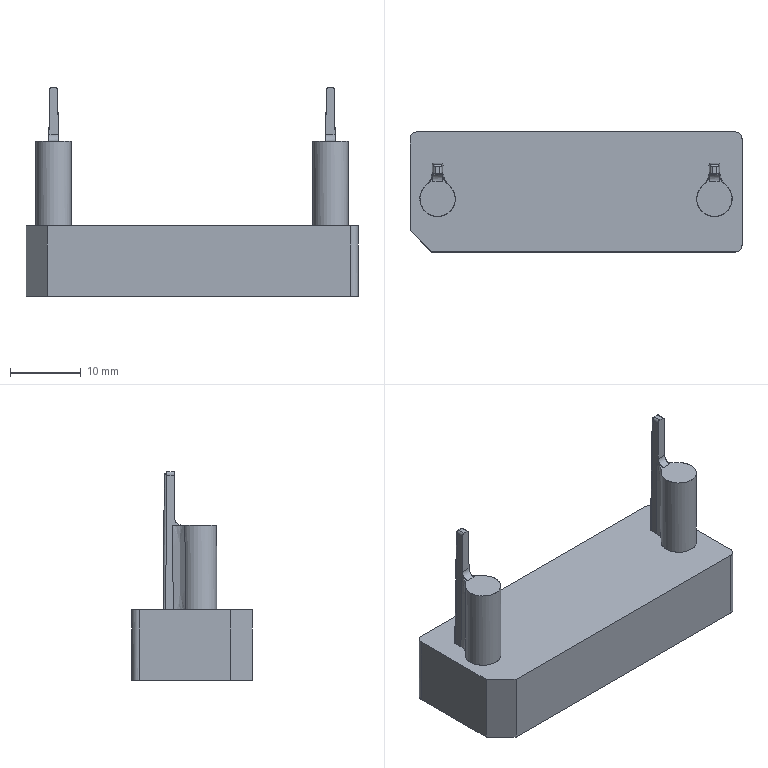NC program | PowerMill | posted with a generic post | part box 47 x 17 x 29.578 mm
Lines 182122 to 182382 of 182382:
N182219 M6
N182220 S15000 M03
N182221 G00 G90 X0.0 Y0.0
N182222 G43 Z10.298 H13
N182223
N182224 G05 P10000 R8
N182225 X-15.205 Y7.6634
N182226 Z-19.73
N182227 G01 Z-19.83 F600.0
N182228 X-14.7025 Y8.0093 F1000.0
N182229 Y5.34
N182230 G00 Z-16.6803
N182231 G01 X-12.9716 Y5.9552 F10000.0
N182232 G00 Z-19.73
N182233 G01 Z-19.83 F600.0
N182234 X-12.9839 Y5.9897 F1000.0
N182235 X-13.0372 Y6.2952
N182236 X-13.0549 Y6.6563
N182237 X-13.0372 Y7.0185
N182238 X-12.9839 Y7.325
N182239 X-12.895 Y7.5757
N182240 X-12.7706 Y7.7707
N182241 X-12.6107 Y7.91
N182242 X-12.4152 Y7.9936
N182243 X-12.1842 Y8.0215
N182244 X-11.9532 Y7.9936
N182245 X-11.7577 Y7.91
N182246 X-11.5977 Y7.7707
N182247 X-11.4733 Y7.5757
N182248 X-11.3845 Y7.325
N182249 X-11.3312 Y7.0185
N182250 X-11.3134 Y6.6563
N182251 X-11.3289 Y6.3236
N182252 X-11.3753 Y6.0369
N182253 X-11.4526 Y5.796
N182254 X-11.5608 Y5.601
N182255 X-11.7 Y5.4519
N182256 X-11.8388 Y5.3649
N182257 X-12.0002 Y5.3126
N182258 X-12.1842 Y5.2952
N182259 X-12.4152 Y5.323
N182260 X-12.6107 Y5.4063
N182261 X-12.7706 Y5.5452
N182262 X-12.895 Y5.7397
N182263 X-12.9716 Y5.9552
N182264 G00 Z-16.6803
N182265 G01 X-9.202 Y6.282 F10000.0
N182266 G00 Z-19.73
N182267 G01 Z-19.83 F600.0
N182268 X-10.2254 F1000.0
N182269 G00 Z-16.6803
N182270 G01 X-5.7356 Y6.1864 F10000.0
N182271 G00 Z-19.73
N182272 G01 Z-19.83 F600.0
N182273 X-5.8267 Y5.9266 F1000.0
N182274 X-5.9563 Y5.7089
N182275 X-6.1242 Y5.5333
N182276 X-6.3313 Y5.401
N182277 X-6.57 Y5.3217
N182278 X-6.8404 Y5.2952
N182279 X-7.1493 Y5.3226
N182280 X-7.4152 Y5.4046
N182281 X-7.6382 Y5.5413
N182282 X-7.8182 Y5.7327
N182283 X-7.9553 Y5.9788
N182284 X-8.0606 Y6.3237
N182285 X-8.0957 Y6.695
N182286 X-8.0712 Y7.019
N182287 X-7.9977 Y7.3008
N182288 X-7.8752 Y7.5404
N182289 X-7.7037 Y7.7379
N182290 X-7.4833 Y7.8933
N182291 X-7.2803 Y7.9837
N182292 X-7.0646 Y8.038
N182293 X-6.8363 Y8.0561
N182294 X-6.5854 Y8.0338
N182295 X-6.3616 Y7.967
N182296 X-6.1649 Y7.8557
N182297 X-6.0001 Y7.7023
N182298 X-5.872 Y7.5093
N182299 X-5.7804 Y7.2768
N182300 G00 Z-16.6803
N182301 G01 X-4.6003 Y7.0716 F10000.0
N182302 G00 Z-19.73
N182303 G01 Z-19.83 F600.0
N182304 X-4.5562 Y7.325 F1000.0
N182305 X-4.4673 Y7.5757
N182306 X-4.3429 Y7.7707
N182307 X-4.183 Y7.91
N182308 X-3.9875 Y7.9936
N182309 X-3.7565 Y8.0215
N182310 X-3.5255 Y7.9936
N182311 X-3.33 Y7.91
N182312 X-3.1701 Y7.7707
N182313 X-3.0457 Y7.5757
N182314 X-2.9568 Y7.325
N182315 X-2.9035 Y7.0185
N182316 X-2.8857 Y6.6563
N182317 X-2.9012 Y6.3236
N182318 X-2.9476 Y6.0369
N182319 X-3.0249 Y5.796
N182320 X-3.1331 Y5.601
N182321 X-3.2723 Y5.4519
N182322 X-3.4111 Y5.3649
N182323 X-3.5725 Y5.3126
N182324 X-3.7565 Y5.2952
N182325 X-3.9875 Y5.323
N182326 X-4.183 Y5.4063
N182327 X-4.3429 Y5.5452
N182328 X-4.4673 Y5.7397
N182329 X-4.5562 Y5.9897
N182330 X-4.6095 Y6.2952
N182331 X-4.6273 Y6.6563
N182332 X-4.6095 Y7.0185
N182333 X-4.6003 Y7.0716
N182334 G00 Z-16.6803
N182335 G01 X-1.0164 Y7.6634 F10000.0
N182336 G00 Z-19.73
N182337 G01 Z-19.83 F600.0
N182338 X-0.5139 Y8.0093 F1000.0
N182339 Y5.34
N182340 G00 Z-16.6803
N182341 G01 X2.1061 Y6.282 F10000.0
N182342 G00 Z-19.73
N182343 G01 Z-19.83 F600.0
N182344 X1.0827 F1000.0
N182345 G00 Z-16.6803
N182346 G01 X4.0405 Y6.7764 F10000.0
N182347 G00 Z-19.73
N182348 G01 Z-19.83 F600.0
N182349 X3.8285 Y6.8026 F1000.0
N182350 X3.6562 Y6.8433
N182351 X3.5237 Y6.8984
N182352 X3.3915 Y7.0063
N182353 X3.3121 Y7.1507
N182354 X3.2857 Y7.3318
N182355 X3.3115 Y7.5221
N182356 X3.3888 Y7.6889
N182357 X3.5176 Y7.8323
N182358 X3.6765 Y7.9374
N182359 X3.8549 Y8.0005
N182360 X4.0527 Y8.0215
N182361 X4.2566 Y8.0009
N182362 X4.437 Y7.9392
N182363 X4.5939 Y7.8363
N182364 X4.7239 Y7.6926
N182365 X4.8018 Y7.5217
N182366 X4.8278 Y7.3236
N182367 X4.7963 Y7.1364
N182368 X4.7019 Y6.988
N182369 X4.5444 Y6.8786
N182370 X4.3239 Y6.808
N182371 X4.0405 Y6.7764
N182372 X4.3176 Y6.7334
N182373 X4.5252 Y6.6859
N182374 X4.6631 Y6.6339
N182375 X4.7832 Y6.5451
N182376 X4.869 Y6.4269
N182377 X4.9205 Y6.2796
N182378 X4.9377 Y6.1029
N182379 X4.909 Y5.8733
N182380 X4.8229 Y5.6752
N182381 X4.6793 Y5.5089
N182382 X4.4998 Y5.3902
N182383 X4.2923 Y5.319
N182384 X4.0568 Y5.2952
N182385 X3.8203 Y5.3194
N182386 X3.6128 Y5.392
N182387 X3.4342 Y5.5129
N182388 X3.2918 Y5.6809
N182389 X3.2063 Y5.881
N182390 X3.1779 Y6.1131
N182391 X3.2063 Y6.3401
N182392 X3.2918 Y6.5137
N182393 X3.4342 Y6.6339
N182394 X3.5622 Y6.6832
N182395 X3.7643 Y6.7307
N182396 X4.0405 Y6.7764
N182397 G00 Z-16.6803
N182398 G01 X7.0349 Y6.282 F10000.0
N182399 G00 Z-19.73
N182400 G01 Z-19.83 F600.0
N182401 X6.0115 F1000.0
N182402 G00 Z-16.6803
N182403 G01 X8.124 Y6.3859 F10000.0
N182404 G00 Z-19.73
N182405 G01 Z-19.83 F600.0
N182406 X8.1107 Y6.6563 F1000.0
N182407 X8.1285 Y7.0185
N182408 X8.1818 Y7.325
N182409 X8.2706 Y7.5757
N182410 X8.395 Y7.7707
N182411 X8.555 Y7.91
N182412 X8.7504 Y7.9936
N182413 X8.9815 Y8.0215
N182414 X9.2125 Y7.9936
N182415 X9.408 Y7.91
N182416 X9.5679 Y7.7707
N182417 X9.6923 Y7.5757
N182418 X9.7811 Y7.325
N182419 X9.8344 Y7.0185
N182420 X9.8522 Y6.6563
N182421 X9.8368 Y6.3236
N182422 X9.7904 Y6.0369
N182423 X9.7131 Y5.796
N182424 X9.6048 Y5.601
N182425 X9.4657 Y5.4519
N182426 X9.3269 Y5.3649
N182427 X9.1655 Y5.3126
N182428 X8.9815 Y5.2952
N182429 X8.7504 Y5.323
N182430 X8.555 Y5.4063
N182431 X8.395 Y5.5452
N182432 X8.2706 Y5.7397
N182433 X8.1818 Y5.9897
N182434 X8.1285 Y6.2952
N182435 X8.124 Y6.3859
N182436 G00 Z-16.6803
N182437 G01 X11.339 Y5.4743 F10000.0
N182438 G00 Z-19.73
N182439 G01 Z-19.83 F600.0
N182440 Y5.8437 F1000.0
N182441 G00 Z-16.6803
N182442 G01 X12.8523 Y7.2484 F10000.0
N182443 G00 Z-19.73
N182444 G01 Z-19.83 F600.0
N182445 X12.8967 Y7.4785 F1000.0
N182446 X12.9838 Y7.6697
N182447 X13.1137 Y7.8221
N182448 X13.282 Y7.9329
N182449 X13.4844 Y7.9993
N182450 X13.721 Y8.0215
N182451 X13.9423 Y8.0002
N182452 X14.1369 Y7.9365
N182453 X14.3049 Y7.8302
N182454 X14.4428 Y7.6776
N182455 X14.5255 Y7.4939
N182456 X14.5531 Y7.2789
N182457 X14.5257 Y7.0998
N182458 X14.4432 Y6.9167
N182459 X14.3239 Y6.7811
N182460 X14.2113 Y6.6726
N182461 X14.1431 Y6.6267
N182462 X14.0332 Y6.5758
N182463 X13.6127 Y6.407
N182464 X13.3726 Y6.2605
N182465 X13.1615 Y6.0806
N182466 X12.973 Y5.8518
N182467 X12.8496 Y5.6049
N182468 X12.7912 Y5.34
N182469 X14.5552
N182470 G00 Z10.298
N182471 G05 P0
N182472 (---------------)
N182473 ( END TOOLPATH : 粗公刻字01-刻字-TEXT_D4 )
N182474 (---------------)
N182475
N182476 M05
N182477 G53 Z0.0
N182478 M30
%